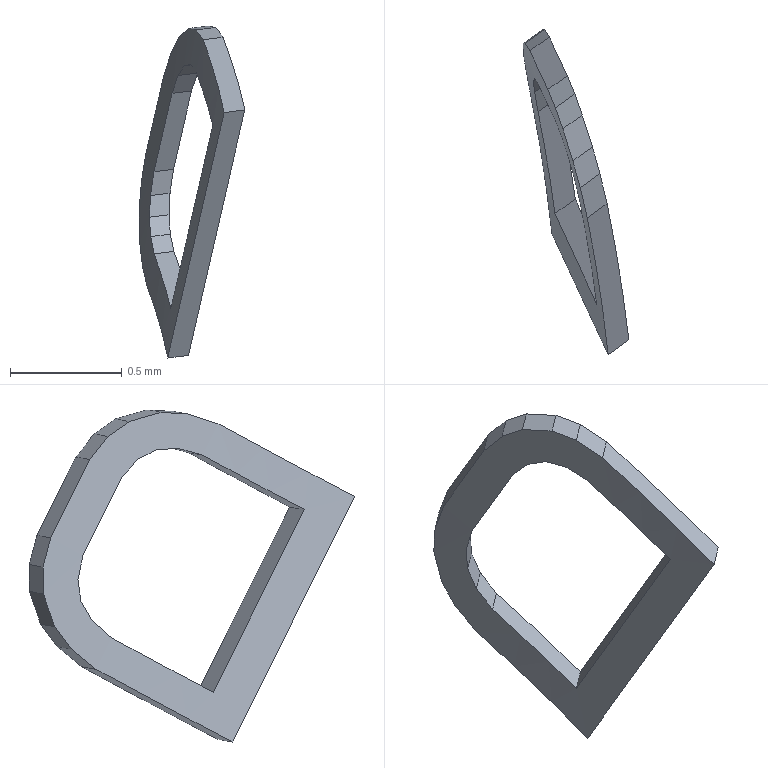Part | SolidWorks | features BaseBody 1 | 1 solid | 28 faces | box 0.4717 x 1.454 x 1.483 mm | volume 0.06327 mm3 | plane 26 | cylinder 2 | commonest cylinder face diameters 16.8 x1 17 x1
STEP:
#1=CARTESIAN_POINT('',(1974.689,-242.141,991.915));
#2=VERTEX_POINT('',#1);
#3=CARTESIAN_POINT('',(1974.596,-241.53,992.24));
#4=VERTEX_POINT('',#3);
#5=CARTESIAN_POINT('',(1966.499,-243.608,993.067));
#6=DIRECTION('',(0.2015,-0.436,0.8771));
#7=DIRECTION('',(-0.7309,-0.6631,-0.1618));
#8=AXIS2_PLACEMENT_3D('',#5,#6,#7);
#9=CIRCLE('',#8,8.4);
#10=EDGE_CURVE('',#2,#4,#9,.T.);
#11=ORIENTED_EDGE('',*,*,#10,.T.);
#12=CARTESIAN_POINT('',(1974.565,-241.396,992.284));
#13=VERTEX_POINT('',#12);
#14=CARTESIAN_POINT('',(1974.596,-241.53,992.24));
#15=CARTESIAN_POINT('',(1974.586,-241.485,992.254));
#16=CARTESIAN_POINT('',(1974.575,-241.44,992.269));
#17=CARTESIAN_POINT('',(1974.565,-241.396,992.284));
#18=B_SPLINE_CURVE_WITH_KNOTS('',3,(#14,#15,#16,#17),.UNSPECIFIED.,.F.,.F.,(4,4),(0.,1.),.UNSPECIFIED.);
#19=EDGE_CURVE('',#4,#13,#18,.T.);
#20=ORIENTED_EDGE('',*,*,#19,.T.);
#21=CARTESIAN_POINT('',(1974.532,-241.275,992.29));
#22=VERTEX_POINT('',#21);
#23=CARTESIAN_POINT('',(1974.565,-241.396,992.284));
#24=CARTESIAN_POINT('',(1974.554,-241.356,992.286));
#25=CARTESIAN_POINT('',(1974.543,-241.315,992.288));
#26=CARTESIAN_POINT('',(1974.532,-241.275,992.29));
#27=B_SPLINE_CURVE_WITH_KNOTS('',3,(#23,#24,#25,#26),.UNSPECIFIED.,.F.,.F.,(4,4),(0.,1.),.UNSPECIFIED.);
#28=EDGE_CURVE('',#13,#22,#27,.T.);
#29=ORIENTED_EDGE('',*,*,#28,.T.);
#30=CARTESIAN_POINT('',(1974.487,-241.133,992.25));
#31=VERTEX_POINT('',#30);
#32=CARTESIAN_POINT('',(1974.532,-241.275,992.29));
#33=CARTESIAN_POINT('',(1974.517,-241.228,992.277));
#34=CARTESIAN_POINT('',(1974.502,-241.18,992.264));
#35=CARTESIAN_POINT('',(1974.487,-241.133,992.25));
#36=B_SPLINE_CURVE_WITH_KNOTS('',3,(#32,#33,#34,#35),.UNSPECIFIED.,.F.,.F.,(4,4),(0.,1.),.UNSPECIFIED.);
#37=EDGE_CURVE('',#22,#31,#36,.T.);
#38=ORIENTED_EDGE('',*,*,#37,.T.);
#39=CARTESIAN_POINT('',(1974.453,-241.039,992.183));
#40=VERTEX_POINT('',#39);
#41=CARTESIAN_POINT('',(1974.487,-241.133,992.25));
#42=CARTESIAN_POINT('',(1974.475,-241.102,992.228));
#43=CARTESIAN_POINT('',(1974.464,-241.07,992.206));
#44=CARTESIAN_POINT('',(1974.453,-241.039,992.183));
#45=B_SPLINE_CURVE_WITH_KNOTS('',3,(#41,#42,#43,#44),.UNSPECIFIED.,.F.,.F.,(4,4),(0.,1.),.UNSPECIFIED.);
#46=EDGE_CURVE('',#31,#40,#45,.T.);
#47=ORIENTED_EDGE('',*,*,#46,.T.);
#48=CARTESIAN_POINT('',(1974.42,-240.957,992.08));
#49=VERTEX_POINT('',#48);
#50=CARTESIAN_POINT('',(1974.453,-241.039,992.183));
#51=CARTESIAN_POINT('',(1974.442,-241.012,992.149));
#52=CARTESIAN_POINT('',(1974.431,-240.984,992.114));
#53=CARTESIAN_POINT('',(1974.42,-240.957,992.08));
#54=B_SPLINE_CURVE_WITH_KNOTS('',3,(#50,#51,#52,#53),.UNSPECIFIED.,.F.,.F.,(4,4),(0.,1.),.UNSPECIFIED.);
#55=EDGE_CURVE('',#40,#49,#54,.T.);
#56=ORIENTED_EDGE('',*,*,#55,.T.);
#57=CARTESIAN_POINT('',(1974.34,-240.783,991.73));
#58=VERTEX_POINT('',#57);
#59=CARTESIAN_POINT('',(1975.457,-243.201,996.593));
#60=DIRECTION('',(-0.2015,0.436,-0.8771));
#61=VECTOR('',#60,1000.);
#62=LINE('',#59,#61);
#63=EDGE_CURVE('',#49,#58,#62,.T.);
#64=ORIENTED_EDGE('',*,*,#63,.T.);
#65=CARTESIAN_POINT('',(1974.319,-240.749,991.6));
#66=VERTEX_POINT('',#65);
#67=CARTESIAN_POINT('',(1974.319,-240.749,991.6));
#68=CARTESIAN_POINT('',(1974.326,-240.76,991.643));
#69=CARTESIAN_POINT('',(1974.333,-240.772,991.687));
#70=CARTESIAN_POINT('',(1974.34,-240.783,991.73));
#71=B_SPLINE_CURVE_WITH_KNOTS('',3,(#67,#68,#69,#70),.UNSPECIFIED.,.F.,.F.,(4,4),(0.,1.),.UNSPECIFIED.);
#72=EDGE_CURVE('',#66,#58,#71,.T.);
#73=ORIENTED_EDGE('',*,*,#72,.F.);
#74=CARTESIAN_POINT('',(1974.31,-240.75,991.48));
#75=VERTEX_POINT('',#74);
#76=CARTESIAN_POINT('',(1974.31,-240.75,991.48));
#77=CARTESIAN_POINT('',(1974.313,-240.75,991.52));
#78=CARTESIAN_POINT('',(1974.316,-240.749,991.56));
#79=CARTESIAN_POINT('',(1974.319,-240.749,991.6));
#80=B_SPLINE_CURVE_WITH_KNOTS('',3,(#76,#77,#78,#79),.UNSPECIFIED.,.F.,.F.,(4,4),(0.,1.),.UNSPECIFIED.);
#81=EDGE_CURVE('',#75,#66,#80,.T.);
#82=ORIENTED_EDGE('',*,*,#81,.F.);
#83=CARTESIAN_POINT('',(1974.312,-240.8,991.334));
#84=VERTEX_POINT('',#83);
#85=CARTESIAN_POINT('',(1974.312,-240.8,991.334));
#86=CARTESIAN_POINT('',(1974.311,-240.783,991.383));
#87=CARTESIAN_POINT('',(1974.311,-240.767,991.431));
#88=CARTESIAN_POINT('',(1974.31,-240.75,991.48));
#89=B_SPLINE_CURVE_WITH_KNOTS('',3,(#85,#86,#87,#88),.UNSPECIFIED.,.F.,.F.,(4,4),(0.,1.),.UNSPECIFIED.);
#90=EDGE_CURVE('',#84,#75,#89,.T.);
#91=ORIENTED_EDGE('',*,*,#90,.F.);
#92=CARTESIAN_POINT('',(1974.323,-240.874,991.234));
#93=VERTEX_POINT('',#92);
#94=CARTESIAN_POINT('',(1974.323,-240.874,991.234));
#95=CARTESIAN_POINT('',(1974.32,-240.849,991.267));
#96=CARTESIAN_POINT('',(1974.316,-240.825,991.3));
#97=CARTESIAN_POINT('',(1974.312,-240.8,991.334));
#98=B_SPLINE_CURVE_WITH_KNOTS('',3,(#94,#95,#96,#97),.UNSPECIFIED.,.F.,.F.,(4,4),(0.,1.),.UNSPECIFIED.);
#99=EDGE_CURVE('',#93,#84,#98,.T.);
#100=ORIENTED_EDGE('',*,*,#99,.F.);
#101=CARTESIAN_POINT('',(1974.344,-240.985,991.144));
#102=VERTEX_POINT('',#101);
#103=CARTESIAN_POINT('',(1974.344,-240.985,991.144));
#104=CARTESIAN_POINT('',(1974.338,-240.948,991.174));
#105=CARTESIAN_POINT('',(1974.331,-240.911,991.204));
#106=CARTESIAN_POINT('',(1974.323,-240.874,991.234));
#107=B_SPLINE_CURVE_WITH_KNOTS('',3,(#103,#104,#105,#106),.UNSPECIFIED.,.F.,.F.,(4,4),(0.,1.),.UNSPECIFIED.);
#108=EDGE_CURVE('',#102,#93,#107,.T.);
#109=ORIENTED_EDGE('',*,*,#108,.F.);
#110=CARTESIAN_POINT('',(1974.437,-241.596,990.818));
#111=VERTEX_POINT('',#110);
#112=CARTESIAN_POINT('',(1966.247,-243.063,991.97));
#113=DIRECTION('',(-0.2015,0.436,-0.8771));
#114=DIRECTION('',(-0.7309,-0.6631,-0.1618));
#115=AXIS2_PLACEMENT_3D('',#112,#113,#114);
#116=CIRCLE('',#115,8.4);
#117=EDGE_CURVE('',#102,#111,#116,.T.);
#118=ORIENTED_EDGE('',*,*,#117,.T.);
#119=CARTESIAN_POINT('',(1975.64,-244.199,996.055));
#120=DIRECTION('',(0.2015,-0.436,0.8771));
#121=VECTOR('',#120,1000.);
#122=LINE('',#119,#121);
#123=EDGE_CURVE('',#111,#2,#122,.T.);
#124=ORIENTED_EDGE('',*,*,#123,.T.);
#125=EDGE_LOOP('',(#11,#20,#29,#38,#47,#56,#64,#73,#82,#91,#100,#109,#118,#124));
#126=FACE_OUTER_BOUND('',#125,.T.);
#127=CARTESIAN_POINT('',(1974.376,-241.055,991.284));
#128=VERTEX_POINT('',#127);
#129=CARTESIAN_POINT('',(1974.361,-240.968,991.36));
#130=VERTEX_POINT('',#129);
#131=CARTESIAN_POINT('',(1974.376,-241.055,991.284));
#132=CARTESIAN_POINT('',(1974.371,-241.026,991.309));
#133=CARTESIAN_POINT('',(1974.366,-240.997,991.335));
#134=CARTESIAN_POINT('',(1974.361,-240.968,991.36));
#135=B_SPLINE_CURVE_WITH_KNOTS('',3,(#131,#132,#133,#134),.UNSPECIFIED.,.F.,.F.,(4,4),(0.,1.),.UNSPECIFIED.);
#136=EDGE_CURVE('',#128,#130,#135,.T.);
#137=ORIENTED_EDGE('',*,*,#136,.T.);
#138=CARTESIAN_POINT('',(1974.355,-240.918,991.447));
#139=VERTEX_POINT('',#138);
#140=CARTESIAN_POINT('',(1974.361,-240.968,991.36));
#141=CARTESIAN_POINT('',(1974.359,-240.951,991.389));
#142=CARTESIAN_POINT('',(1974.357,-240.935,991.418));
#143=CARTESIAN_POINT('',(1974.355,-240.918,991.447));
#144=B_SPLINE_CURVE_WITH_KNOTS('',3,(#140,#141,#142,#143),.UNSPECIFIED.,.F.,.F.,(4,4),(0.,1.),.UNSPECIFIED.);
#145=EDGE_CURVE('',#130,#139,#144,.T.);
#146=ORIENTED_EDGE('',*,*,#145,.T.);
#147=CARTESIAN_POINT('',(1974.36,-240.904,991.544));
#148=VERTEX_POINT('',#147);
#149=CARTESIAN_POINT('',(1974.355,-240.918,991.447));
#150=CARTESIAN_POINT('',(1974.357,-240.913,991.479));
#151=CARTESIAN_POINT('',(1974.359,-240.909,991.512));
#152=CARTESIAN_POINT('',(1974.36,-240.904,991.544));
#153=B_SPLINE_CURVE_WITH_KNOTS('',3,(#149,#150,#151,#152),.UNSPECIFIED.,.F.,.F.,(4,4),(0.,1.),.UNSPECIFIED.);
#154=EDGE_CURVE('',#139,#148,#153,.T.);
#155=ORIENTED_EDGE('',*,*,#154,.T.);
#156=CARTESIAN_POINT('',(1974.376,-240.927,991.65));
#157=VERTEX_POINT('',#156);
#158=CARTESIAN_POINT('',(1974.36,-240.904,991.544));
#159=CARTESIAN_POINT('',(1974.365,-240.912,991.579));
#160=CARTESIAN_POINT('',(1974.371,-240.919,991.615));
#161=CARTESIAN_POINT('',(1974.376,-240.927,991.65));
#162=B_SPLINE_CURVE_WITH_KNOTS('',3,(#158,#159,#160,#161),.UNSPECIFIED.,.F.,.F.,(4,4),(0.,1.),.UNSPECIFIED.);
#163=EDGE_CURVE('',#148,#157,#162,.T.);
#164=ORIENTED_EDGE('',*,*,#163,.T.);
#165=CARTESIAN_POINT('',(1974.456,-241.101,992.));
#166=VERTEX_POINT('',#165);
#167=CARTESIAN_POINT('',(1975.493,-243.344,996.513));
#168=DIRECTION('',(-0.2015,0.436,-0.8771));
#169=VECTOR('',#168,1000.);
#170=LINE('',#167,#169);
#171=EDGE_CURVE('',#166,#157,#170,.T.);
#172=ORIENTED_EDGE('',*,*,#171,.F.);
#173=CARTESIAN_POINT('',(1974.483,-241.171,992.08));
#174=VERTEX_POINT('',#173);
#175=CARTESIAN_POINT('',(1974.483,-241.171,992.08));
#176=CARTESIAN_POINT('',(1974.474,-241.148,992.054));
#177=CARTESIAN_POINT('',(1974.465,-241.124,992.027));
#178=CARTESIAN_POINT('',(1974.456,-241.101,992.));
#179=B_SPLINE_CURVE_WITH_KNOTS('',3,(#175,#176,#177,#178),.UNSPECIFIED.,.F.,.F.,(4,4),(0.,1.),.UNSPECIFIED.);
#180=EDGE_CURVE('',#174,#166,#179,.T.);
#181=ORIENTED_EDGE('',*,*,#180,.F.);
#182=CARTESIAN_POINT('',(1974.511,-241.254,992.124));
#183=VERTEX_POINT('',#182);
#184=CARTESIAN_POINT('',(1974.511,-241.254,992.124));
#185=CARTESIAN_POINT('',(1974.502,-241.227,992.109));
#186=CARTESIAN_POINT('',(1974.493,-241.199,992.095));
#187=CARTESIAN_POINT('',(1974.483,-241.171,992.08));
#188=B_SPLINE_CURVE_WITH_KNOTS('',3,(#184,#185,#186,#187),.UNSPECIFIED.,.F.,.F.,(4,4),(0.,1.),.UNSPECIFIED.);
#189=EDGE_CURVE('',#183,#174,#188,.T.);
#190=ORIENTED_EDGE('',*,*,#189,.F.);
#191=CARTESIAN_POINT('',(1974.538,-241.351,992.13));
#192=VERTEX_POINT('',#191);
#193=CARTESIAN_POINT('',(1974.538,-241.351,992.13));
#194=CARTESIAN_POINT('',(1974.529,-241.318,992.128));
#195=CARTESIAN_POINT('',(1974.52,-241.286,992.126));
#196=CARTESIAN_POINT('',(1974.511,-241.254,992.124));
#197=B_SPLINE_CURVE_WITH_KNOTS('',3,(#193,#194,#195,#196),.UNSPECIFIED.,.F.,.F.,(4,4),(0.,1.),.UNSPECIFIED.);
#198=EDGE_CURVE('',#192,#183,#197,.T.);
#199=ORIENTED_EDGE('',*,*,#198,.F.);
#200=CARTESIAN_POINT('',(1974.564,-241.46,992.1));
#201=VERTEX_POINT('',#200);
#202=CARTESIAN_POINT('',(1974.564,-241.46,992.1));
#203=CARTESIAN_POINT('',(1974.555,-241.424,992.11));
#204=CARTESIAN_POINT('',(1974.547,-241.387,992.12));
#205=CARTESIAN_POINT('',(1974.538,-241.351,992.13));
#206=B_SPLINE_CURVE_WITH_KNOTS('',3,(#202,#203,#204,#205),.UNSPECIFIED.,.F.,.F.,(4,4),(0.,1.),.UNSPECIFIED.);
#207=EDGE_CURVE('',#201,#192,#206,.T.);
#208=ORIENTED_EDGE('',*,*,#207,.F.);
#209=CARTESIAN_POINT('',(1974.639,-241.915,991.857));
#210=VERTEX_POINT('',#209);
#211=CARTESIAN_POINT('',(1966.467,-243.538,992.927));
#212=DIRECTION('',(0.2015,-0.436,0.8771));
#213=DIRECTION('',(-0.7309,-0.6631,-0.1618));
#214=AXIS2_PLACEMENT_3D('',#211,#212,#213);
#215=CIRCLE('',#214,8.4);
#216=EDGE_CURVE('',#210,#201,#215,.T.);
#217=ORIENTED_EDGE('',*,*,#216,.F.);
#218=CARTESIAN_POINT('',(1974.451,-241.509,991.04));
#219=VERTEX_POINT('',#218);
#220=CARTESIAN_POINT('',(1975.622,-244.043,996.137));
#221=DIRECTION('',(0.2015,-0.436,0.8771));
#222=VECTOR('',#221,1000.);
#223=LINE('',#220,#222);
#224=EDGE_CURVE('',#219,#210,#223,.T.);
#225=ORIENTED_EDGE('',*,*,#224,.F.);
#226=CARTESIAN_POINT('',(1966.279,-243.133,992.11));
#227=DIRECTION('',(-0.2015,0.436,-0.8771));
#228=DIRECTION('',(-0.7309,-0.6631,-0.1618));
#229=AXIS2_PLACEMENT_3D('',#226,#227,#228);
#230=CIRCLE('',#229,8.4);
#231=EDGE_CURVE('',#128,#219,#230,.T.);
#232=ORIENTED_EDGE('',*,*,#231,.F.);
#233=EDGE_LOOP('',(#137,#146,#155,#164,#172,#181,#190,#199,#208,#217,#225,#232));
#234=FACE_BOUND('',#233,.T.);
#235=CARTESIAN_POINT('',(1967.45,-245.666,997.207));
#236=DIRECTION('',(0.2015,-0.436,0.8771));
#237=DIRECTION('',(-0.7309,-0.6631,-0.1618));
#238=AXIS2_PLACEMENT_3D('',#235,#236,#237);
#239=CYLINDRICAL_SURFACE('',#238,8.4);
#240=ADVANCED_FACE('',(#126,#234),#239,.F.);
#241=CARTESIAN_POINT('',(1974.782,-242.075,991.926));
#242=VERTEX_POINT('',#241);
#243=CARTESIAN_POINT('',(1974.735,-242.108,991.921));
#244=DIRECTION('',(-0.8088,-0.5792,-0.1022));
#245=VECTOR('',#244,1000.);
#246=LINE('',#243,#245);
#247=EDGE_CURVE('',#242,#2,#246,.T.);
#248=ORIENTED_EDGE('',*,*,#247,.T.);
#249=ORIENTED_EDGE('',*,*,#123,.F.);
#250=CARTESIAN_POINT('',(1974.53,-241.53,990.83));
#251=VERTEX_POINT('',#250);
#252=CARTESIAN_POINT('',(1974.484,-241.563,990.824));
#253=DIRECTION('',(-0.8088,-0.5792,-0.1022));
#254=VECTOR('',#253,1000.);
#255=LINE('',#252,#254);
#256=EDGE_CURVE('',#251,#111,#255,.T.);
#257=ORIENTED_EDGE('',*,*,#256,.F.);
#258=CARTESIAN_POINT('',(1974.656,-241.802,991.378));
#259=DIRECTION('',(0.2015,-0.436,0.8771));
#260=VECTOR('',#259,1000.);
#261=LINE('',#258,#260);
#262=EDGE_CURVE('',#251,#242,#261,.T.);
#263=ORIENTED_EDGE('',*,*,#262,.T.);
#264=EDGE_LOOP('',(#248,#249,#257,#263));
#265=FACE_OUTER_BOUND('',#264,.T.);
#266=CARTESIAN_POINT('',(1980.62,-237.168,991.599));
#267=DIRECTION('',(0.5526,-0.6888,-0.4693));
#268=DIRECTION('',(-0.2015,0.436,-0.8771));
#269=AXIS2_PLACEMENT_3D('',#266,#267,#268);
#270=PLANE('',#269);
#271=ADVANCED_FACE('',(#265),#270,.T.);
#272=ORIENTED_EDGE('',*,*,#256,.T.);
#273=ORIENTED_EDGE('',*,*,#117,.F.);
#274=CARTESIAN_POINT('',(1974.433,-240.922,991.155));
#275=VERTEX_POINT('',#274);
#276=CARTESIAN_POINT('',(1974.388,-240.953,991.149));
#277=DIRECTION('',(-0.8088,-0.5792,-0.1022));
#278=VECTOR('',#277,1000.);
#279=LINE('',#276,#278);
#280=EDGE_CURVE('',#275,#102,#279,.T.);
#281=ORIENTED_EDGE('',*,*,#280,.F.);
#282=CARTESIAN_POINT('',(1966.247,-243.063,991.97));
#283=DIRECTION('',(-0.2015,0.436,-0.8771));
#284=DIRECTION('',(-0.7309,-0.6631,-0.1618));
#285=AXIS2_PLACEMENT_3D('',#282,#283,#284);
#286=CIRCLE('',#285,8.5);
#287=EDGE_CURVE('',#275,#251,#286,.T.);
#288=ORIENTED_EDGE('',*,*,#287,.T.);
#289=EDGE_LOOP('',(#272,#273,#281,#288));
#290=FACE_OUTER_BOUND('',#289,.T.);
#291=CARTESIAN_POINT('',(1981.656,-238.46,990.719));
#292=DIRECTION('',(-0.2015,0.436,-0.8771));
#293=DIRECTION('',(-0.5526,0.6888,0.4693));
#294=AXIS2_PLACEMENT_3D('',#291,#292,#293);
#295=PLANE('',#294);
#296=ADVANCED_FACE('',(#290),#295,.T.);
#297=ORIENTED_EDGE('',*,*,#280,.T.);
#298=ORIENTED_EDGE('',*,*,#108,.T.);
#299=CARTESIAN_POINT('',(1974.411,-240.811,991.245));
#300=VERTEX_POINT('',#299);
#301=CARTESIAN_POINT('',(1974.367,-240.842,991.239));
#302=DIRECTION('',(-0.8088,-0.5792,-0.1022));
#303=VECTOR('',#302,1000.);
#304=LINE('',#301,#303);
#305=EDGE_CURVE('',#300,#93,#304,.T.);
#306=ORIENTED_EDGE('',*,*,#305,.F.);
#307=CARTESIAN_POINT('',(1974.433,-240.922,991.155));
#308=CARTESIAN_POINT('',(1974.428,-240.899,991.173));
#309=CARTESIAN_POINT('',(1974.424,-240.877,991.191));
#310=CARTESIAN_POINT('',(1974.42,-240.855,991.209));
#311=CARTESIAN_POINT('',(1974.416,-240.833,991.227));
#312=CARTESIAN_POINT('',(1974.411,-240.811,991.245));
#313=B_SPLINE_CURVE_WITH_KNOTS('',5,(#307,#308,#309,#310,#311,#312),.UNSPECIFIED.,.F.,.F.,(6,6),(0.,1.),.UNSPECIFIED.);
#314=EDGE_CURVE('',#275,#300,#313,.T.);
#315=ORIENTED_EDGE('',*,*,#314,.F.);
#316=EDGE_LOOP('',(#297,#298,#306,#315));
#317=FACE_OUTER_BOUND('',#316,.T.);
#318=CARTESIAN_POINT('',(1980.208,-236.66,991.977));
#319=DIRECTION('',(-0.308,0.5651,-0.7654));
#320=DIRECTION('',(-0.5011,0.5876,0.6354));
#321=AXIS2_PLACEMENT_3D('',#318,#319,#320);
#322=PLANE('',#321);
#323=ADVANCED_FACE('',(#317),#322,.T.);
#324=ORIENTED_EDGE('',*,*,#305,.T.);
#325=ORIENTED_EDGE('',*,*,#99,.T.);
#326=CARTESIAN_POINT('',(1974.399,-240.737,991.345));
#327=VERTEX_POINT('',#326);
#328=CARTESIAN_POINT('',(1974.356,-240.769,991.339));
#329=DIRECTION('',(-0.8088,-0.5792,-0.1022));
#330=VECTOR('',#329,1000.);
#331=LINE('',#328,#330);
#332=EDGE_CURVE('',#327,#84,#331,.T.);
#333=ORIENTED_EDGE('',*,*,#332,.F.);
#334=CARTESIAN_POINT('',(1974.411,-240.811,991.245));
#335=CARTESIAN_POINT('',(1974.409,-240.796,991.265));
#336=CARTESIAN_POINT('',(1974.407,-240.781,991.285));
#337=CARTESIAN_POINT('',(1974.404,-240.767,991.305));
#338=CARTESIAN_POINT('',(1974.402,-240.752,991.325));
#339=CARTESIAN_POINT('',(1974.399,-240.737,991.345));
#340=B_SPLINE_CURVE_WITH_KNOTS('',5,(#334,#335,#336,#337,#338,#339),.UNSPECIFIED.,.F.,.F.,(6,6),(0.,1.),.UNSPECIFIED.);
#341=EDGE_CURVE('',#300,#327,#340,.T.);
#342=ORIENTED_EDGE('',*,*,#341,.F.);
#343=EDGE_LOOP('',(#324,#325,#333,#342));
#344=FACE_OUTER_BOUND('',#343,.T.);
#345=CARTESIAN_POINT('',(1980.161,-236.611,992.073));
#346=DIRECTION('',(-0.4307,0.7016,-0.5677));
#347=DIRECTION('',(-0.4005,0.4151,0.8169));
#348=AXIS2_PLACEMENT_3D('',#345,#346,#347);
#349=PLANE('',#348);
#350=ADVANCED_FACE('',(#344),#349,.T.);
#351=ORIENTED_EDGE('',*,*,#332,.T.);
#352=ORIENTED_EDGE('',*,*,#90,.T.);
#353=CARTESIAN_POINT('',(1974.397,-240.688,991.491));
#354=VERTEX_POINT('',#353);
#355=CARTESIAN_POINT('',(1974.353,-240.719,991.486));
#356=DIRECTION('',(-0.8088,-0.5792,-0.1022));
#357=VECTOR('',#356,1000.);
#358=LINE('',#355,#357);
#359=EDGE_CURVE('',#354,#75,#358,.T.);
#360=ORIENTED_EDGE('',*,*,#359,.F.);
#361=CARTESIAN_POINT('',(1974.399,-240.737,991.345));
#362=CARTESIAN_POINT('',(1974.399,-240.727,991.374));
#363=CARTESIAN_POINT('',(1974.398,-240.718,991.403));
#364=CARTESIAN_POINT('',(1974.398,-240.708,991.433));
#365=CARTESIAN_POINT('',(1974.397,-240.698,991.462));
#366=CARTESIAN_POINT('',(1974.397,-240.688,991.491));
#367=B_SPLINE_CURVE_WITH_KNOTS('',5,(#361,#362,#363,#364,#365,#366),.UNSPECIFIED.,.F.,.F.,(6,6),(0.,1.),.UNSPECIFIED.);
#368=EDGE_CURVE('',#327,#354,#367,.T.);
#369=ORIENTED_EDGE('',*,*,#368,.F.);
#370=EDGE_LOOP('',(#351,#352,#360,#369));
#371=FACE_OUTER_BOUND('',#370,.T.);
#372=CARTESIAN_POINT('',(1980.125,-236.586,992.215));
#373=DIRECTION('',(-0.5358,0.7972,-0.2783));
#374=DIRECTION('',(-0.2426,0.1703,0.955));
#375=AXIS2_PLACEMENT_3D('',#372,#373,#374);
#376=PLANE('',#375);
#377=ADVANCED_FACE('',(#371),#376,.T.);
#378=ORIENTED_EDGE('',*,*,#359,.T.);
#379=ORIENTED_EDGE('',*,*,#81,.T.);
#380=CARTESIAN_POINT('',(1974.406,-240.687,991.611));
#381=VERTEX_POINT('',#380);
#382=CARTESIAN_POINT('',(1974.362,-240.718,991.606));
#383=DIRECTION('',(-0.8088,-0.5792,-0.1022));
#384=VECTOR('',#383,1000.);
#385=LINE('',#382,#384);
#386=EDGE_CURVE('',#381,#66,#385,.T.);
#387=ORIENTED_EDGE('',*,*,#386,.F.);
#388=CARTESIAN_POINT('',(1974.397,-240.688,991.491));
#389=CARTESIAN_POINT('',(1974.399,-240.688,991.515));
#390=CARTESIAN_POINT('',(1974.4,-240.688,991.539));
#391=CARTESIAN_POINT('',(1974.402,-240.687,991.563));
#392=CARTESIAN_POINT('',(1974.404,-240.687,991.587));
#393=CARTESIAN_POINT('',(1974.406,-240.687,991.611));
#394=B_SPLINE_CURVE_WITH_KNOTS('',5,(#388,#389,#390,#391,#392,#393),.UNSPECIFIED.,.F.,.F.,(6,6),(0.,1.),.UNSPECIFIED.);
#395=EDGE_CURVE('',#354,#381,#394,.T.);
#396=ORIENTED_EDGE('',*,*,#395,.F.);
#397=EDGE_LOOP('',(#378,#379,#387,#396));
#398=FACE_OUTER_BOUND('',#397,.T.);
#399=CARTESIAN_POINT('',(1980.117,-236.596,992.333));
#400=DIRECTION('',(-0.5849,0.8103,0.03586));
#401=DIRECTION('',(-0.06203,-0.08877,0.9941));
#402=AXIS2_PLACEMENT_3D('',#399,#400,#401);
#403=PLANE('',#402);
#404=ADVANCED_FACE('',(#398),#403,.T.);
#405=ORIENTED_EDGE('',*,*,#386,.T.);
#406=ORIENTED_EDGE('',*,*,#72,.T.);
#407=CARTESIAN_POINT('',(1974.426,-240.721,991.741));
#408=VERTEX_POINT('',#407);
#409=CARTESIAN_POINT('',(1974.383,-240.752,991.736));
#410=DIRECTION('',(-0.8088,-0.5792,-0.1022));
#411=VECTOR('',#410,1000.);
#412=LINE('',#409,#411);
#413=EDGE_CURVE('',#408,#58,#412,.T.);
#414=ORIENTED_EDGE('',*,*,#413,.F.);
#415=CARTESIAN_POINT('',(1974.406,-240.687,991.611));
#416=CARTESIAN_POINT('',(1974.41,-240.694,991.637));
#417=CARTESIAN_POINT('',(1974.414,-240.701,991.663));
#418=CARTESIAN_POINT('',(1974.418,-240.707,991.689));
#419=CARTESIAN_POINT('',(1974.422,-240.714,991.715));
#420=CARTESIAN_POINT('',(1974.426,-240.721,991.741));
#421=B_SPLINE_CURVE_WITH_KNOTS('',5,(#415,#416,#417,#418,#419,#420),.UNSPECIFIED.,.F.,.F.,(6,6),(0.,1.),.UNSPECIFIED.);
#422=EDGE_CURVE('',#381,#408,#421,.T.);
#423=ORIENTED_EDGE('',*,*,#422,.F.);
#424=EDGE_LOOP('',(#405,#406,#414,#423));
#425=FACE_OUTER_BOUND('',#424,.T.);
#426=CARTESIAN_POINT('',(1980.13,-236.636,992.462));
#427=DIRECTION('',(-0.581,0.7597,0.292));
#428=DIRECTION('',(0.09152,-0.2955,0.9509));
#429=AXIS2_PLACEMENT_3D('',#426,#427,#428);
#430=PLANE('',#429);
#431=ADVANCED_FACE('',(#425),#430,.T.);
#432=ORIENTED_EDGE('',*,*,#413,.T.);
#433=ORIENTED_EDGE('',*,*,#63,.F.);
#434=CARTESIAN_POINT('',(1974.506,-240.895,992.091));
#435=VERTEX_POINT('',#434);
#436=CARTESIAN_POINT('',(1974.463,-240.926,992.085));
#437=DIRECTION('',(-0.8088,-0.5792,-0.1022));
#438=VECTOR('',#437,1000.);
#439=LINE('',#436,#438);
#440=EDGE_CURVE('',#435,#49,#439,.T.);
#441=ORIENTED_EDGE('',*,*,#440,.F.);
#442=CARTESIAN_POINT('',(1974.466,-240.808,991.916));
#443=DIRECTION('',(-0.2015,0.436,-0.8771));
#444=VECTOR('',#443,1000.);
#445=LINE('',#442,#444);
#446=EDGE_CURVE('',#435,#408,#445,.T.);
#447=ORIENTED_EDGE('',*,*,#446,.T.);
#448=EDGE_LOOP('',(#432,#433,#441,#447));
#449=FACE_OUTER_BOUND('',#448,.T.);
#450=CARTESIAN_POINT('',(1980.21,-236.81,992.812));
#451=DIRECTION('',(-0.5526,0.6888,0.4693));
#452=DIRECTION('',(0.2015,-0.436,0.8771));
#453=AXIS2_PLACEMENT_3D('',#450,#451,#452);
#454=PLANE('',#453);
#455=ADVANCED_FACE('',(#449),#454,.T.);
#456=ORIENTED_EDGE('',*,*,#440,.T.);
#457=ORIENTED_EDGE('',*,*,#55,.F.);
#458=CARTESIAN_POINT('',(1974.54,-240.977,992.194));
#459=VERTEX_POINT('',#458);
#460=CARTESIAN_POINT('',(1974.496,-241.008,992.189));
#461=DIRECTION('',(-0.8088,-0.5792,-0.1022));
#462=VECTOR('',#461,1000.);
#463=LINE('',#460,#462);
#464=EDGE_CURVE('',#459,#40,#463,.T.);
#465=ORIENTED_EDGE('',*,*,#464,.F.);
#466=CARTESIAN_POINT('',(1974.54,-240.977,992.194));
#467=CARTESIAN_POINT('',(1974.533,-240.96,992.174));
#468=CARTESIAN_POINT('',(1974.526,-240.944,992.153));
#469=CARTESIAN_POINT('',(1974.52,-240.928,992.132));
#470=CARTESIAN_POINT('',(1974.513,-240.911,992.112));
#471=CARTESIAN_POINT('',(1974.506,-240.895,992.091));
#472=B_SPLINE_CURVE_WITH_KNOTS('',5,(#466,#467,#468,#469,#470,#471),.UNSPECIFIED.,.F.,.F.,(6,6),(0.,1.),.UNSPECIFIED.);
#473=EDGE_CURVE('',#459,#435,#472,.T.);
#474=ORIENTED_EDGE('',*,*,#473,.T.);
#475=EDGE_LOOP('',(#456,#457,#465,#474));
#476=FACE_OUTER_BOUND('',#475,.T.);
#477=CARTESIAN_POINT('',(1980.251,-236.886,992.916));
#478=DIRECTION('',(-0.5035,0.5921,0.6292));
#479=DIRECTION('',(0.3039,-0.5603,0.7705));
#480=AXIS2_PLACEMENT_3D('',#477,#478,#479);
#481=PLANE('',#480);
#482=ADVANCED_FACE('',(#476),#481,.T.);
#483=ORIENTED_EDGE('',*,*,#464,.T.);
#484=ORIENTED_EDGE('',*,*,#46,.F.);
#485=CARTESIAN_POINT('',(1974.574,-241.071,992.261));
#486=VERTEX_POINT('',#485);
#487=CARTESIAN_POINT('',(1974.53,-241.102,992.256));
#488=DIRECTION('',(-0.8088,-0.5792,-0.1022));
#489=VECTOR('',#488,1000.);
#490=LINE('',#487,#489);
#491=EDGE_CURVE('',#486,#31,#490,.T.);
#492=ORIENTED_EDGE('',*,*,#491,.F.);
#493=CARTESIAN_POINT('',(1974.574,-241.071,992.261));
#494=CARTESIAN_POINT('',(1974.567,-241.052,992.248));
#495=CARTESIAN_POINT('',(1974.56,-241.033,992.234));
#496=CARTESIAN_POINT('',(1974.553,-241.014,992.221));
#497=CARTESIAN_POINT('',(1974.546,-240.996,992.208));
#498=CARTESIAN_POINT('',(1974.54,-240.977,992.194));
#499=B_SPLINE_CURVE_WITH_KNOTS('',5,(#493,#494,#495,#496,#497,#498),.UNSPECIFIED.,.F.,.F.,(6,6),(0.,1.),.UNSPECIFIED.);
#500=EDGE_CURVE('',#486,#459,#499,.T.);
#501=ORIENTED_EDGE('',*,*,#500,.T.);
#502=EDGE_LOOP('',(#483,#484,#492,#501));
#503=FACE_OUTER_BOUND('',#502,.T.);
#504=CARTESIAN_POINT('',(1980.301,-236.969,992.985));
#505=DIRECTION('',(-0.4077,0.4269,0.8072));
#506=DIRECTION('',(0.4239,-0.6945,0.5814));
#507=AXIS2_PLACEMENT_3D('',#504,#505,#506);
#508=PLANE('',#507);
#509=ADVANCED_FACE('',(#503),#508,.T.);
#510=ORIENTED_EDGE('',*,*,#491,.T.);
#511=ORIENTED_EDGE('',*,*,#37,.F.);
#512=CARTESIAN_POINT('',(1974.619,-241.213,992.301));
#513=VERTEX_POINT('',#512);
#514=CARTESIAN_POINT('',(1974.575,-241.244,992.296));
#515=DIRECTION('',(-0.8088,-0.5792,-0.1022));
#516=VECTOR('',#515,1000.);
#517=LINE('',#514,#516);
#518=EDGE_CURVE('',#513,#22,#517,.T.);
#519=ORIENTED_EDGE('',*,*,#518,.F.);
#520=CARTESIAN_POINT('',(1974.619,-241.213,992.301));
#521=CARTESIAN_POINT('',(1974.61,-241.184,992.293));
#522=CARTESIAN_POINT('',(1974.601,-241.156,992.285));
#523=CARTESIAN_POINT('',(1974.592,-241.128,992.277));
#524=CARTESIAN_POINT('',(1974.583,-241.099,992.269));
#525=CARTESIAN_POINT('',(1974.574,-241.071,992.261));
#526=B_SPLINE_CURVE_WITH_KNOTS('',5,(#520,#521,#522,#523,#524,#525),.UNSPECIFIED.,.F.,.F.,(6,6),(0.,1.),.UNSPECIFIED.);
#527=EDGE_CURVE('',#513,#486,#526,.T.);
#528=ORIENTED_EDGE('',*,*,#527,.T.);
#529=EDGE_LOOP('',(#510,#511,#519,#528));
#530=FACE_OUTER_BOUND('',#529,.T.);
#531=CARTESIAN_POINT('',(1980.38,-237.087,993.029));
#532=DIRECTION('',(-0.2539,0.1871,0.949));
#533=DIRECTION('',(0.5305,-0.7934,0.2983));
#534=AXIS2_PLACEMENT_3D('',#531,#532,#533);
#535=PLANE('',#534);
#536=ADVANCED_FACE('',(#530),#535,.T.);
#537=ORIENTED_EDGE('',*,*,#518,.T.);
#538=ORIENTED_EDGE('',*,*,#28,.F.);
#539=CARTESIAN_POINT('',(1974.652,-241.333,992.295));
#540=VERTEX_POINT('',#539);
#541=CARTESIAN_POINT('',(1974.609,-241.364,992.289));
#542=DIRECTION('',(-0.8088,-0.5792,-0.1022));
#543=VECTOR('',#542,1000.);
#544=LINE('',#541,#543);
#545=EDGE_CURVE('',#540,#13,#544,.T.);
#546=ORIENTED_EDGE('',*,*,#545,.F.);
#547=CARTESIAN_POINT('',(1974.652,-241.333,992.295));
#548=CARTESIAN_POINT('',(1974.646,-241.309,992.296));
#549=CARTESIAN_POINT('',(1974.639,-241.285,992.297));
#550=CARTESIAN_POINT('',(1974.633,-241.261,992.299));
#551=CARTESIAN_POINT('',(1974.626,-241.237,992.3));
#552=CARTESIAN_POINT('',(1974.619,-241.213,992.301));
#553=B_SPLINE_CURVE_WITH_KNOTS('',5,(#547,#548,#549,#550,#551,#552),.UNSPECIFIED.,.F.,.F.,(6,6),(0.,1.),.UNSPECIFIED.);
#554=EDGE_CURVE('',#540,#513,#553,.T.);
#555=ORIENTED_EDGE('',*,*,#554,.T.);
#556=EDGE_LOOP('',(#537,#538,#546,#555));
#557=FACE_OUTER_BOUND('',#556,.T.);
#558=CARTESIAN_POINT('',(1980.449,-237.182,993.027));
#559=DIRECTION('',(-0.07187,-0.07511,0.9946));
#560=DIRECTION('',(0.5837,-0.8117,-0.01912));
#561=AXIS2_PLACEMENT_3D('',#558,#559,#560);
#562=PLANE('',#561);
#563=ADVANCED_FACE('',(#557),#562,.T.);
#564=ORIENTED_EDGE('',*,*,#545,.T.);
#565=ORIENTED_EDGE('',*,*,#19,.F.);
#566=CARTESIAN_POINT('',(1974.684,-241.467,992.251));
#567=VERTEX_POINT('',#566);
#568=CARTESIAN_POINT('',(1974.64,-241.498,992.246));
#569=DIRECTION('',(-0.8088,-0.5792,-0.1022));
#570=VECTOR('',#569,1000.);
#571=LINE('',#568,#570);
#572=EDGE_CURVE('',#567,#4,#571,.T.);
#573=ORIENTED_EDGE('',*,*,#572,.F.);
#574=CARTESIAN_POINT('',(1974.684,-241.467,992.251));
#575=CARTESIAN_POINT('',(1974.678,-241.44,992.26));
#576=CARTESIAN_POINT('',(1974.672,-241.413,992.269));
#577=CARTESIAN_POINT('',(1974.666,-241.386,992.277));
#578=CARTESIAN_POINT('',(1974.659,-241.36,992.286));
#579=CARTESIAN_POINT('',(1974.652,-241.333,992.295));
#580=B_SPLINE_CURVE_WITH_KNOTS('',5,(#574,#575,#576,#577,#578,#579),.UNSPECIFIED.,.F.,.F.,(6,6),(0.,1.),.UNSPECIFIED.);
#581=EDGE_CURVE('',#567,#540,#580,.T.);
#582=ORIENTED_EDGE('',*,*,#581,.T.);
#583=EDGE_LOOP('',(#564,#565,#573,#582));
#584=FACE_OUTER_BOUND('',#583,.T.);
#585=CARTESIAN_POINT('',(1980.526,-237.283,992.989));
#586=DIRECTION('',(0.08681,-0.2894,0.9533));
#587=DIRECTION('',(0.5817,-0.7621,-0.2843));
#588=AXIS2_PLACEMENT_3D('',#585,#586,#587);
#589=PLANE('',#588);
#590=ADVANCED_FACE('',(#584),#589,.T.);
#591=ORIENTED_EDGE('',*,*,#572,.T.);
#592=ORIENTED_EDGE('',*,*,#10,.F.);
#593=ORIENTED_EDGE('',*,*,#247,.F.);
#594=CARTESIAN_POINT('',(1966.499,-243.608,993.067));
#595=DIRECTION('',(0.2015,-0.436,0.8771));
#596=DIRECTION('',(-0.7309,-0.6631,-0.1618));
#597=AXIS2_PLACEMENT_3D('',#594,#595,#596);
#598=CIRCLE('',#597,8.5);
#599=EDGE_CURVE('',#242,#567,#598,.T.);
#600=ORIENTED_EDGE('',*,*,#599,.T.);
#601=EDGE_LOOP('',(#591,#592,#593,#600));
#602=FACE_OUTER_BOUND('',#601,.T.);
#603=CARTESIAN_POINT('',(1982.253,-239.435,991.522));
#604=DIRECTION('',(0.2015,-0.436,0.8771));
#605=DIRECTION('',(0.5526,-0.6888,-0.4693));
#606=AXIS2_PLACEMENT_3D('',#603,#604,#605);
#607=PLANE('',#606);
#608=ADVANCED_FACE('',(#602),#607,.T.);
#609=CARTESIAN_POINT('',(1974.465,-240.991,991.295));
#610=VERTEX_POINT('',#609);
#611=CARTESIAN_POINT('',(1974.542,-241.444,991.052));
#612=VERTEX_POINT('',#611);
#613=CARTESIAN_POINT('',(1966.279,-243.133,992.11));
#614=DIRECTION('',(-0.2015,0.436,-0.8771));
#615=DIRECTION('',(-0.7309,-0.6631,-0.1618));
#616=AXIS2_PLACEMENT_3D('',#613,#614,#615);
#617=CIRCLE('',#616,8.5);
#618=EDGE_CURVE('',#610,#612,#617,.T.);
#619=ORIENTED_EDGE('',*,*,#618,.F.);
#620=CARTESIAN_POINT('',(1974.42,-241.023,991.289));
#621=DIRECTION('',(-0.8088,-0.5792,-0.1022));
#622=VECTOR('',#621,1000.);
#623=LINE('',#620,#622);
#624=EDGE_CURVE('',#610,#128,#623,.T.);
#625=ORIENTED_EDGE('',*,*,#624,.T.);
#626=ORIENTED_EDGE('',*,*,#231,.T.);
#627=CARTESIAN_POINT('',(1974.497,-241.476,991.046));
#628=DIRECTION('',(-0.8088,-0.5792,-0.1022));
#629=VECTOR('',#628,1000.);
#630=LINE('',#627,#629);
#631=EDGE_CURVE('',#612,#219,#630,.T.);
#632=ORIENTED_EDGE('',*,*,#631,.F.);
#633=EDGE_LOOP('',(#619,#625,#626,#632));
#634=FACE_OUTER_BOUND('',#633,.T.);
#635=CARTESIAN_POINT('',(1981.688,-238.529,990.859));
#636=DIRECTION('',(-0.2015,0.436,-0.8771));
#637=DIRECTION('',(-0.5526,0.6888,0.4693));
#638=AXIS2_PLACEMENT_3D('',#635,#636,#637);
#639=PLANE('',#638);
#640=ADVANCED_FACE('',(#634),#639,.F.);
#641=CARTESIAN_POINT('',(1974.73,-241.85,991.868));
#642=VERTEX_POINT('',#641);
#643=CARTESIAN_POINT('',(1974.636,-241.647,991.46));
#644=DIRECTION('',(0.2015,-0.436,0.8771));
#645=VECTOR('',#644,1000.);
#646=LINE('',#643,#645);
#647=EDGE_CURVE('',#612,#642,#646,.T.);
#648=ORIENTED_EDGE('',*,*,#647,.F.);
#649=ORIENTED_EDGE('',*,*,#631,.T.);
#650=ORIENTED_EDGE('',*,*,#224,.T.);
#651=CARTESIAN_POINT('',(1974.684,-241.882,991.863));
#652=DIRECTION('',(-0.8088,-0.5792,-0.1022));
#653=VECTOR('',#652,1000.);
#654=LINE('',#651,#653);
#655=EDGE_CURVE('',#642,#210,#654,.T.);
#656=ORIENTED_EDGE('',*,*,#655,.F.);
#657=EDGE_LOOP('',(#648,#649,#650,#656));
#658=FACE_OUTER_BOUND('',#657,.T.);
#659=CARTESIAN_POINT('',(1980.565,-237.13,991.813));
#660=DIRECTION('',(0.5526,-0.6888,-0.4693));
#661=DIRECTION('',(-0.2015,0.436,-0.8771));
#662=AXIS2_PLACEMENT_3D('',#659,#660,#661);
#663=PLANE('',#662);
#664=ADVANCED_FACE('',(#658),#663,.F.);
#665=CARTESIAN_POINT('',(1974.652,-241.397,992.111));
#666=VERTEX_POINT('',#665);
#667=CARTESIAN_POINT('',(1966.467,-243.538,992.927));
#668=DIRECTION('',(0.2015,-0.436,0.8771));
#669=DIRECTION('',(-0.7309,-0.6631,-0.1618));
#670=AXIS2_PLACEMENT_3D('',#667,#668,#669);
#671=CIRCLE('',#670,8.5);
#672=EDGE_CURVE('',#642,#666,#671,.T.);
#673=ORIENTED_EDGE('',*,*,#672,.F.);
#674=ORIENTED_EDGE('',*,*,#655,.T.);
#675=ORIENTED_EDGE('',*,*,#216,.T.);
#676=CARTESIAN_POINT('',(1974.608,-241.429,992.106));
#677=DIRECTION('',(-0.8088,-0.5792,-0.1022));
#678=VECTOR('',#677,1000.);
#679=LINE('',#676,#678);
#680=EDGE_CURVE('',#666,#201,#679,.T.);
#681=ORIENTED_EDGE('',*,*,#680,.F.);
#682=EDGE_LOOP('',(#673,#674,#675,#681));
#683=FACE_OUTER_BOUND('',#682,.T.);
#684=CARTESIAN_POINT('',(1982.134,-239.258,991.456));
#685=DIRECTION('',(0.2015,-0.436,0.8771));
#686=DIRECTION('',(0.5526,-0.6888,-0.4693));
#687=AXIS2_PLACEMENT_3D('',#684,#685,#686);
#688=PLANE('',#687);
#689=ADVANCED_FACE('',(#683),#688,.F.);
#690=CARTESIAN_POINT('',(1974.626,-241.288,992.141));
#691=VERTEX_POINT('',#690);
#692=CARTESIAN_POINT('',(1974.652,-241.397,992.111));
#693=CARTESIAN_POINT('',(1974.647,-241.375,992.117));
#694=CARTESIAN_POINT('',(1974.642,-241.353,992.123));
#695=CARTESIAN_POINT('',(1974.637,-241.331,992.129));
#696=CARTESIAN_POINT('',(1974.631,-241.309,992.135));
#697=CARTESIAN_POINT('',(1974.626,-241.288,992.141));
#698=B_SPLINE_CURVE_WITH_KNOTS('',5,(#692,#693,#694,#695,#696,#697),.UNSPECIFIED.,.F.,.F.,(6,6),(0.,1.),.UNSPECIFIED.);
#699=EDGE_CURVE('',#666,#691,#698,.T.);
#700=ORIENTED_EDGE('',*,*,#699,.F.);
#701=ORIENTED_EDGE('',*,*,#680,.T.);
#702=ORIENTED_EDGE('',*,*,#207,.T.);
#703=CARTESIAN_POINT('',(1974.582,-241.319,992.136));
#704=DIRECTION('',(-0.8088,-0.5792,-0.1022));
#705=VECTOR('',#704,1000.);
#706=LINE('',#703,#705);
#707=EDGE_CURVE('',#691,#192,#706,.T.);
#708=ORIENTED_EDGE('',*,*,#707,.F.);
#709=EDGE_LOOP('',(#700,#701,#702,#708));
#710=FACE_OUTER_BOUND('',#709,.T.);
#711=CARTESIAN_POINT('',(1980.494,-237.213,992.849));
#712=DIRECTION('',(0.05851,-0.2521,0.9659));
#713=DIRECTION('',(0.5852,-0.7752,-0.2378));
#714=AXIS2_PLACEMENT_3D('',#711,#712,#713);
#715=PLANE('',#714);
#716=ADVANCED_FACE('',(#710),#715,.F.);
#717=CARTESIAN_POINT('',(1974.598,-241.192,992.135));
#718=VERTEX_POINT('',#717);
#719=CARTESIAN_POINT('',(1974.626,-241.288,992.141));
#720=CARTESIAN_POINT('',(1974.62,-241.268,992.14));
#721=CARTESIAN_POINT('',(1974.615,-241.249,992.139));
#722=CARTESIAN_POINT('',(1974.609,-241.23,992.137));
#723=CARTESIAN_POINT('',(1974.604,-241.211,992.136));
#724=CARTESIAN_POINT('',(1974.598,-241.192,992.135));
#725=B_SPLINE_CURVE_WITH_KNOTS('',5,(#719,#720,#721,#722,#723,#724),.UNSPECIFIED.,.F.,.F.,(6,6),(0.,1.),.UNSPECIFIED.);
#726=EDGE_CURVE('',#691,#718,#725,.T.);
#727=ORIENTED_EDGE('',*,*,#726,.F.);
#728=ORIENTED_EDGE('',*,*,#707,.T.);
#729=ORIENTED_EDGE('',*,*,#198,.T.);
#730=CARTESIAN_POINT('',(1974.555,-241.223,992.129));
#731=DIRECTION('',(-0.8088,-0.5792,-0.1022));
#732=VECTOR('',#731,1000.);
#733=LINE('',#730,#732);
#734=EDGE_CURVE('',#718,#183,#733,.T.);
#735=ORIENTED_EDGE('',*,*,#734,.F.);
#736=EDGE_LOOP('',(#727,#728,#729,#735));
#737=FACE_OUTER_BOUND('',#736,.T.);
#738=CARTESIAN_POINT('',(1980.431,-237.13,992.875));
#739=DIRECTION('',(-0.1444,0.0272,0.9891));
#740=DIRECTION('',(0.5701,-0.8147,0.1057));
#741=AXIS2_PLACEMENT_3D('',#738,#739,#740);
#742=PLANE('',#741);
#743=ADVANCED_FACE('',(#737),#742,.F.);
#744=CARTESIAN_POINT('',(1974.571,-241.109,992.091));
#745=VERTEX_POINT('',#744);
#746=CARTESIAN_POINT('',(1974.598,-241.192,992.135));
#747=CARTESIAN_POINT('',(1974.593,-241.175,992.126));
#748=CARTESIAN_POINT('',(1974.587,-241.158,992.117));
#749=CARTESIAN_POINT('',(1974.582,-241.142,992.109));
#750=CARTESIAN_POINT('',(1974.576,-241.125,992.1));
#751=CARTESIAN_POINT('',(1974.571,-241.109,992.091));
#752=B_SPLINE_CURVE_WITH_KNOTS('',5,(#746,#747,#748,#749,#750,#751),.UNSPECIFIED.,.F.,.F.,(6,6),(0.,1.),.UNSPECIFIED.);
#753=EDGE_CURVE('',#718,#745,#752,.T.);
#754=ORIENTED_EDGE('',*,*,#753,.F.);
#755=ORIENTED_EDGE('',*,*,#734,.T.);
#756=ORIENTED_EDGE('',*,*,#189,.T.);
#757=CARTESIAN_POINT('',(1974.527,-241.14,992.086));
#758=DIRECTION('',(-0.8088,-0.5792,-0.1022));
#759=VECTOR('',#758,1000.);
#760=LINE('',#757,#759);
#761=EDGE_CURVE('',#745,#174,#760,.T.);
#762=ORIENTED_EDGE('',*,*,#761,.F.);
#763=EDGE_LOOP('',(#754,#755,#756,#762));
#764=FACE_OUTER_BOUND('',#763,.T.);
#765=CARTESIAN_POINT('',(1980.377,-237.053,992.865));
#766=DIRECTION('',(-0.3526,0.3384,0.8724));
#767=DIRECTION('',(0.4707,-0.7416,0.4779));
#768=AXIS2_PLACEMENT_3D('',#765,#766,#767);
#769=PLANE('',#768);
#770=ADVANCED_FACE('',(#764),#769,.F.);
#771=CARTESIAN_POINT('',(1974.543,-241.038,992.011));
#772=VERTEX_POINT('',#771);
#773=CARTESIAN_POINT('',(1974.571,-241.109,992.091));
#774=CARTESIAN_POINT('',(1974.565,-241.094,992.075));
#775=CARTESIAN_POINT('',(1974.56,-241.08,992.059));
#776=CARTESIAN_POINT('',(1974.554,-241.066,992.043));
#777=CARTESIAN_POINT('',(1974.549,-241.052,992.027));
#778=CARTESIAN_POINT('',(1974.543,-241.038,992.011));
#779=B_SPLINE_CURVE_WITH_KNOTS('',5,(#773,#774,#775,#776,#777,#778),.UNSPECIFIED.,.F.,.F.,(6,6),(0.,1.),.UNSPECIFIED.);
#780=EDGE_CURVE('',#745,#772,#779,.T.);
#781=ORIENTED_EDGE('',*,*,#780,.F.);
#782=ORIENTED_EDGE('',*,*,#761,.T.);
#783=ORIENTED_EDGE('',*,*,#180,.T.);
#784=CARTESIAN_POINT('',(1974.5,-241.069,992.006));
#785=DIRECTION('',(-0.8088,-0.5792,-0.1022));
#786=VECTOR('',#785,1000.);
#787=LINE('',#784,#786);
#788=EDGE_CURVE('',#772,#166,#787,.T.);
#789=ORIENTED_EDGE('',*,*,#788,.F.);
#790=EDGE_LOOP('',(#781,#782,#783,#789));
#791=FACE_OUTER_BOUND('',#790,.T.);
#792=CARTESIAN_POINT('',(1980.332,-236.982,992.819));
#793=DIRECTION('',(-0.4888,0.5653,0.6644));
#794=DIRECTION('',(0.3271,-0.5873,0.7403));
#795=AXIS2_PLACEMENT_3D('',#792,#793,#794);
#796=PLANE('',#795);
#797=ADVANCED_FACE('',(#791),#796,.F.);
#798=CARTESIAN_POINT('',(1974.463,-240.864,991.661));
#799=VERTEX_POINT('',#798);
#800=CARTESIAN_POINT('',(1974.503,-240.951,991.836));
#801=DIRECTION('',(-0.2015,0.436,-0.8771));
#802=VECTOR('',#801,1000.);
#803=LINE('',#800,#802);
#804=EDGE_CURVE('',#772,#799,#803,.T.);
#805=ORIENTED_EDGE('',*,*,#804,.F.);
#806=ORIENTED_EDGE('',*,*,#788,.T.);
#807=ORIENTED_EDGE('',*,*,#171,.T.);
#808=CARTESIAN_POINT('',(1974.419,-240.895,991.656));
#809=DIRECTION('',(-0.8088,-0.5792,-0.1022));
#810=VECTOR('',#809,1000.);
#811=LINE('',#808,#810);
#812=EDGE_CURVE('',#799,#157,#811,.T.);
#813=ORIENTED_EDGE('',*,*,#812,.F.);
#814=EDGE_LOOP('',(#805,#806,#807,#813));
#815=FACE_OUTER_BOUND('',#814,.T.);
#816=CARTESIAN_POINT('',(1980.296,-236.918,992.738));
#817=DIRECTION('',(-0.5526,0.6888,0.4693));
#818=DIRECTION('',(0.2015,-0.436,0.8771));
#819=AXIS2_PLACEMENT_3D('',#816,#817,#818);
#820=PLANE('',#819);
#821=ADVANCED_FACE('',(#815),#820,.F.);
#822=CARTESIAN_POINT('',(1974.448,-240.842,991.555));
#823=VERTEX_POINT('',#822);
#824=CARTESIAN_POINT('',(1974.448,-240.842,991.555));
#825=CARTESIAN_POINT('',(1974.451,-240.846,991.576));
#826=CARTESIAN_POINT('',(1974.454,-240.851,991.597));
#827=CARTESIAN_POINT('',(1974.457,-240.855,991.619));
#828=CARTESIAN_POINT('',(1974.46,-240.86,991.64));
#829=CARTESIAN_POINT('',(1974.463,-240.864,991.661));
#830=B_SPLINE_CURVE_WITH_KNOTS('',5,(#824,#825,#826,#827,#828,#829),.UNSPECIFIED.,.F.,.F.,(6,6),(0.,1.),.UNSPECIFIED.);
#831=EDGE_CURVE('',#823,#799,#830,.T.);
#832=ORIENTED_EDGE('',*,*,#831,.T.);
#833=ORIENTED_EDGE('',*,*,#812,.T.);
#834=ORIENTED_EDGE('',*,*,#163,.F.);
#835=CARTESIAN_POINT('',(1974.404,-240.873,991.549));
#836=DIRECTION('',(-0.8088,-0.5792,-0.1022));
#837=VECTOR('',#836,1000.);
#838=LINE('',#835,#837);
#839=EDGE_CURVE('',#823,#148,#838,.T.);
#840=ORIENTED_EDGE('',*,*,#839,.F.);
#841=EDGE_LOOP('',(#832,#833,#834,#840));
#842=FACE_OUTER_BOUND('',#841,.T.);
#843=CARTESIAN_POINT('',(1980.216,-236.744,992.388));
#844=DIRECTION('',(-0.5846,0.7727,0.2473));
#845=DIRECTION('',(0.0643,-0.2598,0.9635));
#846=AXIS2_PLACEMENT_3D('',#843,#844,#845);
#847=PLANE('',#846);
#848=ADVANCED_FACE('',(#842),#847,.F.);
#849=CARTESIAN_POINT('',(1974.443,-240.855,991.458));
#850=VERTEX_POINT('',#849);
#851=CARTESIAN_POINT('',(1974.443,-240.855,991.458));
#852=CARTESIAN_POINT('',(1974.444,-240.853,991.478));
#853=CARTESIAN_POINT('',(1974.445,-240.85,991.497));
#854=CARTESIAN_POINT('',(1974.446,-240.847,991.516));
#855=CARTESIAN_POINT('',(1974.447,-240.844,991.536));
#856=CARTESIAN_POINT('',(1974.448,-240.842,991.555));
#857=B_SPLINE_CURVE_WITH_KNOTS('',5,(#851,#852,#853,#854,#855,#856),.UNSPECIFIED.,.F.,.F.,(6,6),(0.,1.),.UNSPECIFIED.);
#858=EDGE_CURVE('',#850,#823,#857,.T.);
#859=ORIENTED_EDGE('',*,*,#858,.T.);
#860=ORIENTED_EDGE('',*,*,#839,.T.);
#861=ORIENTED_EDGE('',*,*,#154,.F.);
#862=CARTESIAN_POINT('',(1974.399,-240.887,991.453));
#863=DIRECTION('',(-0.8088,-0.5792,-0.1022));
#864=VECTOR('',#863,1000.);
#865=LINE('',#862,#864);
#866=EDGE_CURVE('',#850,#139,#865,.T.);
#867=ORIENTED_EDGE('',*,*,#866,.F.);
#868=EDGE_LOOP('',(#859,#860,#861,#867));
#869=FACE_OUTER_BOUND('',#868,.T.);
#870=CARTESIAN_POINT('',(1980.209,-236.716,992.283));
#871=DIRECTION('',(-0.5728,0.8151,-0.08642));
#872=DIRECTION('',(-0.1333,0.01136,0.991));
#873=AXIS2_PLACEMENT_3D('',#870,#871,#872);
#874=PLANE('',#873);
#875=ADVANCED_FACE('',(#869),#874,.F.);
#876=CARTESIAN_POINT('',(1974.449,-240.905,991.372));
#877=VERTEX_POINT('',#876);
#878=CARTESIAN_POINT('',(1974.449,-240.905,991.372));
#879=CARTESIAN_POINT('',(1974.448,-240.895,991.389));
#880=CARTESIAN_POINT('',(1974.447,-240.885,991.406));
#881=CARTESIAN_POINT('',(1974.445,-240.875,991.424));
#882=CARTESIAN_POINT('',(1974.444,-240.865,991.441));
#883=CARTESIAN_POINT('',(1974.443,-240.855,991.458));
#884=B_SPLINE_CURVE_WITH_KNOTS('',5,(#878,#879,#880,#881,#882,#883),.UNSPECIFIED.,.F.,.F.,(6,6),(0.,1.),.UNSPECIFIED.);
#885=EDGE_CURVE('',#877,#850,#884,.T.);
#886=ORIENTED_EDGE('',*,*,#885,.T.);
#887=ORIENTED_EDGE('',*,*,#866,.T.);
#888=ORIENTED_EDGE('',*,*,#145,.F.);
#889=CARTESIAN_POINT('',(1974.405,-240.936,991.366));
#890=DIRECTION('',(-0.8088,-0.5792,-0.1022));
#891=VECTOR('',#890,1000.);
#892=LINE('',#889,#891);
#893=EDGE_CURVE('',#877,#130,#892,.T.);
#894=ORIENTED_EDGE('',*,*,#893,.F.);
#895=EDGE_LOOP('',(#886,#887,#888,#894));
#896=FACE_OUTER_BOUND('',#895,.T.);
#897=CARTESIAN_POINT('',(1980.222,-236.717,992.188));
#898=DIRECTION('',(-0.4775,0.7481,-0.4609));
#899=DIRECTION('',(-0.3434,0.3239,0.8816));
#900=AXIS2_PLACEMENT_3D('',#897,#898,#899);
#901=PLANE('',#900);
#902=ADVANCED_FACE('',(#896),#901,.F.);
#903=CARTESIAN_POINT('',(1974.465,-240.991,991.295));
#904=CARTESIAN_POINT('',(1974.462,-240.974,991.31));
#905=CARTESIAN_POINT('',(1974.459,-240.957,991.325));
#906=CARTESIAN_POINT('',(1974.455,-240.939,991.341));
#907=CARTESIAN_POINT('',(1974.452,-240.922,991.356));
#908=CARTESIAN_POINT('',(1974.449,-240.905,991.372));
#909=B_SPLINE_CURVE_WITH_KNOTS('',5,(#903,#904,#905,#906,#907,#908),.UNSPECIFIED.,.F.,.F.,(6,6),(0.,1.),.UNSPECIFIED.);
#910=EDGE_CURVE('',#610,#877,#909,.T.);
#911=ORIENTED_EDGE('',*,*,#910,.T.);
#912=ORIENTED_EDGE('',*,*,#893,.T.);
#913=ORIENTED_EDGE('',*,*,#136,.F.);
#914=ORIENTED_EDGE('',*,*,#624,.F.);
#915=EDGE_LOOP('',(#911,#912,#913,#914));
#916=FACE_OUTER_BOUND('',#915,.T.);
#917=CARTESIAN_POINT('',(1980.254,-236.747,992.105));
#918=DIRECTION('',(-0.3319,0.5929,-0.7337));
#919=DIRECTION('',(-0.4855,0.5595,0.6717));
#920=AXIS2_PLACEMENT_3D('',#917,#918,#919);
#921=PLANE('',#920);
#922=ADVANCED_FACE('',(#916),#921,.F.);
#923=ORIENTED_EDGE('',*,*,#262,.F.);
#924=ORIENTED_EDGE('',*,*,#287,.F.);
#925=ORIENTED_EDGE('',*,*,#314,.T.);
#926=ORIENTED_EDGE('',*,*,#341,.T.);
#927=ORIENTED_EDGE('',*,*,#368,.T.);
#928=ORIENTED_EDGE('',*,*,#395,.T.);
#929=ORIENTED_EDGE('',*,*,#422,.T.);
#930=ORIENTED_EDGE('',*,*,#446,.F.);
#931=ORIENTED_EDGE('',*,*,#473,.F.);
#932=ORIENTED_EDGE('',*,*,#500,.F.);
#933=ORIENTED_EDGE('',*,*,#527,.F.);
#934=ORIENTED_EDGE('',*,*,#554,.F.);
#935=ORIENTED_EDGE('',*,*,#581,.F.);
#936=ORIENTED_EDGE('',*,*,#599,.F.);
#937=EDGE_LOOP('',(#923,#924,#925,#926,#927,#928,#929,#930,#931,#932,#933,#934,#935,#936));
#938=FACE_OUTER_BOUND('',#937,.T.);
#939=ORIENTED_EDGE('',*,*,#672,.T.);
#940=ORIENTED_EDGE('',*,*,#699,.T.);
#941=ORIENTED_EDGE('',*,*,#726,.T.);
#942=ORIENTED_EDGE('',*,*,#753,.T.);
#943=ORIENTED_EDGE('',*,*,#780,.T.);
#944=ORIENTED_EDGE('',*,*,#804,.T.);
#945=ORIENTED_EDGE('',*,*,#831,.F.);
#946=ORIENTED_EDGE('',*,*,#858,.F.);
#947=ORIENTED_EDGE('',*,*,#885,.F.);
#948=ORIENTED_EDGE('',*,*,#910,.F.);
#949=ORIENTED_EDGE('',*,*,#618,.T.);
#950=ORIENTED_EDGE('',*,*,#647,.T.);
#951=EDGE_LOOP('',(#939,#940,#941,#942,#943,#944,#945,#946,#947,#948,#949,#950));
#952=FACE_BOUND('',#951,.T.);
#953=CARTESIAN_POINT('',(1967.45,-245.666,997.207));
#954=DIRECTION('',(0.2015,-0.436,0.8771));
#955=DIRECTION('',(-0.7309,-0.6631,-0.1618));
#956=AXIS2_PLACEMENT_3D('',#953,#954,#955);
#957=CYLINDRICAL_SURFACE('',#956,8.5);
#958=ADVANCED_FACE('',(#938,#952),#957,.T.);
#959=CLOSED_SHELL('',(#240,#271,#296,#323,#350,#377,#404,#431,#455,#482,#509,#536,#563,#590,#608,#640,#664,#689,#716,#743,#770,#797,#821,#848,#875,#902,#922,#958));
#960=MANIFOLD_SOLID_BREP('',#959);
#961=CARTESIAN_POINT('',(0.,0.,0.));
#962=DIRECTION('',(0.,0.,1.));
#963=DIRECTION('',(1.,0.,0.));
#964=AXIS2_PLACEMENT_3D('',#961,#962,#963);
#965=(LENGTH_UNIT()NAMED_UNIT(*)SI_UNIT(.MILLI.,.METRE.));
#966=UNCERTAINTY_MEASURE_WITH_UNIT(LENGTH_MEASURE(0.00001),#965,'','');
#967=(NAMED_UNIT(*)PLANE_ANGLE_UNIT()SI_UNIT($,.RADIAN.));
#968=(NAMED_UNIT(*)SI_UNIT($,.STERADIAN.)SOLID_ANGLE_UNIT());
#969=(GEOMETRIC_REPRESENTATION_CONTEXT(3)GLOBAL_UNCERTAINTY_ASSIGNED_CONTEXT((#966))GLOBAL_UNIT_ASSIGNED_CONTEXT((#965,#967,#968))REPRESENTATION_CONTEXT('',''));
#970=ADVANCED_BREP_SHAPE_REPRESENTATION('',(#960,#964),#969);